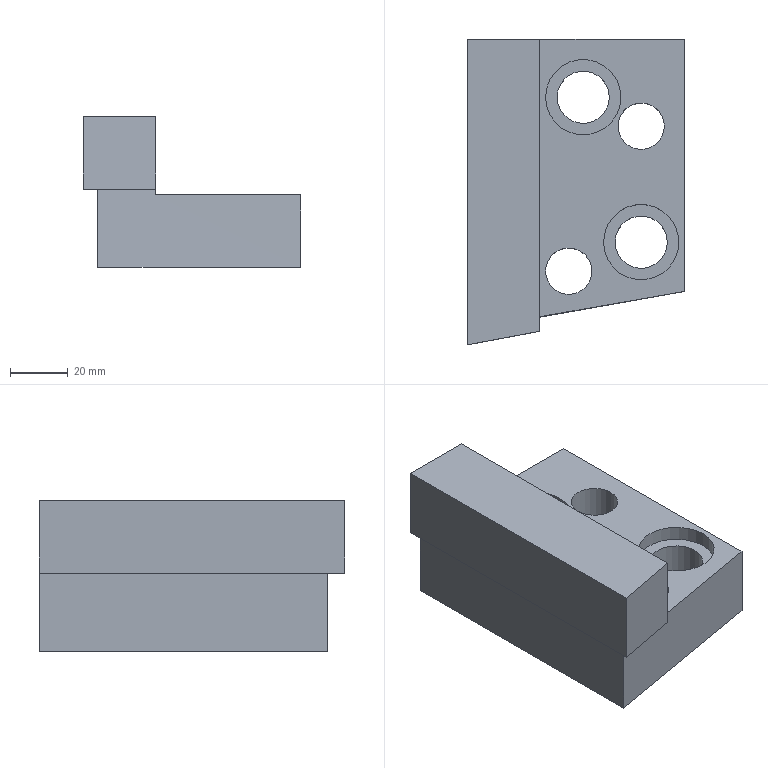Part | NX | features solid 2 | 1 solid | 19 faces | box 75 x 105.467 x 52 mm | volume 205777 mm3 | plane 11 | cylinder 6 | spline 2 | commonest cylinder face diameters 16 x2 18 x2 26 x2
STEP:
#1=CARTESIAN_POINT('',(-221.,545.,-55.));
#2=VERTEX_POINT('',#1);
#3=CARTESIAN_POINT('',(-230.,545.,-55.));
#4=DIRECTION('',(0.,0.,1.));
#5=DIRECTION('',(1.,0.,0.));
#6=AXIS2_PLACEMENT_3D('',#3,#4,#5);
#7=CIRCLE('',#6,9.);
#8=EDGE_CURVE('',#2,#2,#7,.F.);
#9=ORIENTED_EDGE('',*,*,#8,.F.);
#10=EDGE_LOOP('',(#9));
#11=FACE_BOUND('',#10,.T.);
#12=CARTESIAN_POINT('',(-241.,595.,-55.));
#13=VERTEX_POINT('',#12);
#14=CARTESIAN_POINT('',(-250.,595.,-55.));
#15=DIRECTION('',(0.,0.,1.));
#16=DIRECTION('',(1.,0.,0.));
#17=AXIS2_PLACEMENT_3D('',#14,#15,#16);
#18=CIRCLE('',#17,9.);
#19=EDGE_CURVE('',#13,#13,#18,.T.);
#20=ORIENTED_EDGE('',*,*,#19,.T.);
#21=EDGE_LOOP('',(#20));
#22=FACE_BOUND('',#21,.T.);
#23=CARTESIAN_POINT('',(-222.,585.,-55.));
#24=VERTEX_POINT('',#23);
#25=CARTESIAN_POINT('',(-230.,585.,-55.));
#26=DIRECTION('',(0.,0.,1.));
#27=DIRECTION('',(1.,0.,0.));
#28=AXIS2_PLACEMENT_3D('',#25,#26,#27);
#29=CIRCLE('',#28,8.);
#30=EDGE_CURVE('',#24,#24,#29,.T.);
#31=ORIENTED_EDGE('',*,*,#30,.T.);
#32=EDGE_LOOP('',(#31));
#33=FACE_BOUND('',#32,.T.);
#34=CARTESIAN_POINT('',(-215.,528.003,-55.));
#35=VERTEX_POINT('',#34);
#36=CARTESIAN_POINT('',(-215.,615.,-55.));
#37=VERTEX_POINT('',#36);
#38=CARTESIAN_POINT('',(-215.,477.364,-55.));
#39=DIRECTION('',(0.,1.,0.));
#40=VECTOR('',#39,1000.);
#41=LINE('',#38,#40);
#42=EDGE_CURVE('',#35,#37,#41,.T.);
#43=ORIENTED_EDGE('',*,*,#42,.F.);
#44=CARTESIAN_POINT('',(-285.,515.602,-55.));
#45=VERTEX_POINT('',#44);
#46=CARTESIAN_POINT('',(-215.,528.003,-55.));
#47=CARTESIAN_POINT('',(-226.671,525.962,-55.));
#48=CARTESIAN_POINT('',(-250.01,521.86,-55.));
#49=CARTESIAN_POINT('',(-273.364,517.836,-55.));
#50=CARTESIAN_POINT('',(-285.,515.602,-55.));
#51=B_SPLINE_CURVE_WITH_KNOTS('',3,(#46,#47,#48,#49,#50),.UNSPECIFIED.,.F.,.F.,(4,1,4),(0.,0.03555,0.07109),.UNSPECIFIED.);
#52=EDGE_CURVE('',#35,#45,#51,.T.);
#53=ORIENTED_EDGE('',*,*,#52,.T.);
#54=CARTESIAN_POINT('',(-285.,615.,-55.));
#55=VERTEX_POINT('',#54);
#56=CARTESIAN_POINT('',(-285.,474.207,-55.));
#57=DIRECTION('',(0.,1.,0.));
#58=VECTOR('',#57,1000.);
#59=LINE('',#56,#58);
#60=EDGE_CURVE('',#45,#55,#59,.T.);
#61=ORIENTED_EDGE('',*,*,#60,.T.);
#62=CARTESIAN_POINT('',(-277.501,615.,-55.));
#63=DIRECTION('',(-1.,0.,0.));
#64=VECTOR('',#63,1000.);
#65=LINE('',#62,#64);
#66=EDGE_CURVE('',#37,#55,#65,.T.);
#67=ORIENTED_EDGE('',*,*,#66,.F.);
#68=EDGE_LOOP('',(#43,#53,#61,#67));
#69=FACE_BOUND('',#68,.T.);
#70=CARTESIAN_POINT('',(-247.,535.,-55.));
#71=VERTEX_POINT('',#70);
#72=CARTESIAN_POINT('',(-255.,535.,-55.));
#73=DIRECTION('',(0.,0.,1.));
#74=DIRECTION('',(1.,0.,0.));
#75=AXIS2_PLACEMENT_3D('',#72,#73,#74);
#76=CIRCLE('',#75,8.);
#77=EDGE_CURVE('',#71,#71,#76,.F.);
#78=ORIENTED_EDGE('',*,*,#77,.F.);
#79=EDGE_LOOP('',(#78));
#80=FACE_BOUND('',#79,.T.);
#81=CARTESIAN_POINT('',(-277.501,477.364,-55.));
#82=DIRECTION('',(0.,0.,1.));
#83=DIRECTION('',(1.,0.,0.));
#84=AXIS2_PLACEMENT_3D('',#81,#82,#83);
#85=PLANE('',#84);
#86=ADVANCED_FACE('',(#11,#22,#33,#69,#80),#85,.F.);
#87=CARTESIAN_POINT('',(-217.,545.,-30.));
#88=VERTEX_POINT('',#87);
#89=CARTESIAN_POINT('',(-230.,545.,-30.));
#90=DIRECTION('',(0.,0.,1.));
#91=DIRECTION('',(1.,0.,0.));
#92=AXIS2_PLACEMENT_3D('',#89,#90,#91);
#93=CIRCLE('',#92,13.);
#94=EDGE_CURVE('',#88,#88,#93,.F.);
#95=ORIENTED_EDGE('',*,*,#94,.T.);
#96=EDGE_LOOP('',(#95));
#97=FACE_BOUND('',#96,.T.);
#98=CARTESIAN_POINT('',(-215.,528.003,-30.));
#99=VERTEX_POINT('',#98);
#100=CARTESIAN_POINT('',(-265.,519.259,-30.));
#101=VERTEX_POINT('',#100);
#102=CARTESIAN_POINT('',(-215.,528.003,-30.));
#103=CARTESIAN_POINT('',(-231.667,525.088,-30.));
#104=CARTESIAN_POINT('',(-248.333,522.174,-30.));
#105=CARTESIAN_POINT('',(-265.,519.259,-30.));
#106=B_SPLINE_CURVE_WITH_KNOTS('',3,(#102,#103,#104,#105),.UNSPECIFIED.,.F.,.F.,(4,4),(0.,0.05076),.UNSPECIFIED.);
#107=EDGE_CURVE('',#99,#101,#106,.T.);
#108=ORIENTED_EDGE('',*,*,#107,.F.);
#109=CARTESIAN_POINT('',(-215.,615.,-30.));
#110=VERTEX_POINT('',#109);
#111=CARTESIAN_POINT('',(-215.,487.395,-30.));
#112=DIRECTION('',(0.,1.,0.));
#113=VECTOR('',#112,1000.);
#114=LINE('',#111,#113);
#115=EDGE_CURVE('',#99,#110,#114,.T.);
#116=ORIENTED_EDGE('',*,*,#115,.T.);
#117=CARTESIAN_POINT('',(-265.,615.,-30.));
#118=VERTEX_POINT('',#117);
#119=CARTESIAN_POINT('',(-237.5,615.,-30.));
#120=DIRECTION('',(-1.,0.,0.));
#121=VECTOR('',#120,1000.);
#122=LINE('',#119,#121);
#123=EDGE_CURVE('',#110,#118,#122,.T.);
#124=ORIENTED_EDGE('',*,*,#123,.T.);
#125=CARTESIAN_POINT('',(-265.,487.395,-30.));
#126=DIRECTION('',(0.,1.,0.));
#127=VECTOR('',#126,1000.);
#128=LINE('',#125,#127);
#129=EDGE_CURVE('',#101,#118,#128,.T.);
#130=ORIENTED_EDGE('',*,*,#129,.F.);
#131=EDGE_LOOP('',(#108,#116,#124,#130));
#132=FACE_BOUND('',#131,.T.);
#133=CARTESIAN_POINT('',(-222.,585.,-30.));
#134=VERTEX_POINT('',#133);
#135=CARTESIAN_POINT('',(-230.,585.,-30.));
#136=DIRECTION('',(0.,0.,1.));
#137=DIRECTION('',(1.,0.,0.));
#138=AXIS2_PLACEMENT_3D('',#135,#136,#137);
#139=CIRCLE('',#138,8.);
#140=EDGE_CURVE('',#134,#134,#139,.T.);
#141=ORIENTED_EDGE('',*,*,#140,.F.);
#142=EDGE_LOOP('',(#141));
#143=FACE_BOUND('',#142,.T.);
#144=CARTESIAN_POINT('',(-237.,595.,-30.));
#145=VERTEX_POINT('',#144);
#146=CARTESIAN_POINT('',(-250.,595.,-30.));
#147=DIRECTION('',(0.,0.,1.));
#148=DIRECTION('',(1.,0.,0.));
#149=AXIS2_PLACEMENT_3D('',#146,#147,#148);
#150=CIRCLE('',#149,13.);
#151=EDGE_CURVE('',#145,#145,#150,.T.);
#152=ORIENTED_EDGE('',*,*,#151,.F.);
#153=EDGE_LOOP('',(#152));
#154=FACE_BOUND('',#153,.T.);
#155=CARTESIAN_POINT('',(-247.,535.,-30.));
#156=VERTEX_POINT('',#155);
#157=CARTESIAN_POINT('',(-255.,535.,-30.));
#158=DIRECTION('',(0.,0.,1.));
#159=DIRECTION('',(1.,0.,0.));
#160=AXIS2_PLACEMENT_3D('',#157,#158,#159);
#161=CIRCLE('',#160,8.);
#162=EDGE_CURVE('',#156,#156,#161,.F.);
#163=ORIENTED_EDGE('',*,*,#162,.T.);
#164=EDGE_LOOP('',(#163));
#165=FACE_BOUND('',#164,.T.);
#166=CARTESIAN_POINT('',(-237.5,487.395,-30.));
#167=DIRECTION('',(0.,0.,1.));
#168=DIRECTION('',(1.,0.,0.));
#169=AXIS2_PLACEMENT_3D('',#166,#167,#168);
#170=PLANE('',#169);
#171=ADVANCED_FACE('',(#97,#132,#143,#154,#165),#170,.T.);
#172=CARTESIAN_POINT('',(-217.,545.,-35.));
#173=VERTEX_POINT('',#172);
#174=CARTESIAN_POINT('',(-230.,545.,-35.));
#175=DIRECTION('',(0.,0.,1.));
#176=DIRECTION('',(1.,0.,0.));
#177=AXIS2_PLACEMENT_3D('',#174,#175,#176);
#178=CIRCLE('',#177,13.);
#179=EDGE_CURVE('',#173,#173,#178,.T.);
#180=ORIENTED_EDGE('',*,*,#179,.T.);
#181=EDGE_LOOP('',(#180));
#182=FACE_BOUND('',#181,.T.);
#183=CARTESIAN_POINT('',(-221.,545.,-35.));
#184=VERTEX_POINT('',#183);
#185=CARTESIAN_POINT('',(-230.,545.,-35.));
#186=DIRECTION('',(0.,0.,1.));
#187=DIRECTION('',(1.,0.,0.));
#188=AXIS2_PLACEMENT_3D('',#185,#186,#187);
#189=CIRCLE('',#188,9.);
#190=EDGE_CURVE('',#184,#184,#189,.F.);
#191=ORIENTED_EDGE('',*,*,#190,.T.);
#192=EDGE_LOOP('',(#191));
#193=FACE_BOUND('',#192,.T.);
#194=CARTESIAN_POINT('',(-230.,545.,-35.));
#195=DIRECTION('',(0.,0.,1.));
#196=DIRECTION('',(1.,0.,0.));
#197=AXIS2_PLACEMENT_3D('',#194,#195,#196);
#198=PLANE('',#197);
#199=ADVANCED_FACE('',(#182,#193),#198,.T.);
#200=CARTESIAN_POINT('',(-290.,509.533,-3.));
#201=VERTEX_POINT('',#200);
#202=CARTESIAN_POINT('',(-290.,509.533,-28.));
#203=VERTEX_POINT('',#202);
#204=CARTESIAN_POINT('',(-290.,509.533,100.));
#205=DIRECTION('',(0.,0.,-1.));
#206=VECTOR('',#205,1000.);
#207=LINE('',#204,#206);
#208=EDGE_CURVE('',#201,#203,#207,.T.);
#209=ORIENTED_EDGE('',*,*,#208,.F.);
#210=CARTESIAN_POINT('',(-290.,615.,-3.));
#211=VERTEX_POINT('',#210);
#212=CARTESIAN_POINT('',(-290.,474.207,-3.));
#213=DIRECTION('',(0.,1.,0.));
#214=VECTOR('',#213,1000.);
#215=LINE('',#212,#214);
#216=EDGE_CURVE('',#201,#211,#215,.T.);
#217=ORIENTED_EDGE('',*,*,#216,.T.);
#218=CARTESIAN_POINT('',(-290.,615.,-28.));
#219=VERTEX_POINT('',#218);
#220=CARTESIAN_POINT('',(-290.,615.,-53.));
#221=DIRECTION('',(0.,0.,1.));
#222=VECTOR('',#221,1000.);
#223=LINE('',#220,#222);
#224=EDGE_CURVE('',#219,#211,#223,.T.);
#225=ORIENTED_EDGE('',*,*,#224,.F.);
#226=CARTESIAN_POINT('',(-290.,474.207,-28.));
#227=DIRECTION('',(0.,-1.,0.));
#228=VECTOR('',#227,1000.);
#229=LINE('',#226,#228);
#230=EDGE_CURVE('',#203,#219,#229,.F.);
#231=ORIENTED_EDGE('',*,*,#230,.F.);
#232=EDGE_LOOP('',(#209,#217,#225,#231));
#233=FACE_BOUND('',#232,.T.);
#234=CARTESIAN_POINT('',(-290.,474.207,-53.));
#235=DIRECTION('',(1.,0.,0.));
#236=DIRECTION('',(0.,0.,-1.));
#237=AXIS2_PLACEMENT_3D('',#234,#235,#236);
#238=PLANE('',#237);
#239=ADVANCED_FACE('',(#233),#238,.F.);
#240=CARTESIAN_POINT('',(-265.,519.259,-28.));
#241=VERTEX_POINT('',#240);
#242=CARTESIAN_POINT('',(-265.,514.183,-28.));
#243=VERTEX_POINT('',#242);
#244=CARTESIAN_POINT('',(-265.,480.509,-28.));
#245=DIRECTION('',(0.,-1.,0.));
#246=VECTOR('',#245,1000.);
#247=LINE('',#244,#246);
#248=EDGE_CURVE('',#241,#243,#247,.T.);
#249=ORIENTED_EDGE('',*,*,#248,.F.);
#250=CARTESIAN_POINT('',(-265.,519.259,-78.));
#251=DIRECTION('',(0.,0.,-1.));
#252=VECTOR('',#251,1000.);
#253=LINE('',#250,#252);
#254=EDGE_CURVE('',#101,#241,#253,.F.);
#255=ORIENTED_EDGE('',*,*,#254,.F.);
#256=ORIENTED_EDGE('',*,*,#129,.T.);
#257=CARTESIAN_POINT('',(-265.,615.,-3.));
#258=VERTEX_POINT('',#257);
#259=CARTESIAN_POINT('',(-265.,615.,-53.));
#260=DIRECTION('',(0.,0.,1.));
#261=VECTOR('',#260,1000.);
#262=LINE('',#259,#261);
#263=EDGE_CURVE('',#118,#258,#262,.T.);
#264=ORIENTED_EDGE('',*,*,#263,.T.);
#265=CARTESIAN_POINT('',(-265.,514.183,-3.));
#266=VERTEX_POINT('',#265);
#267=CARTESIAN_POINT('',(-265.,480.509,-3.));
#268=DIRECTION('',(0.,1.,0.));
#269=VECTOR('',#268,1000.);
#270=LINE('',#267,#269);
#271=EDGE_CURVE('',#266,#258,#270,.T.);
#272=ORIENTED_EDGE('',*,*,#271,.F.);
#273=CARTESIAN_POINT('',(-265.,514.183,100.));
#274=DIRECTION('',(0.,0.,-1.));
#275=VECTOR('',#274,1000.);
#276=LINE('',#273,#275);
#277=EDGE_CURVE('',#266,#243,#276,.T.);
#278=ORIENTED_EDGE('',*,*,#277,.T.);
#279=EDGE_LOOP('',(#249,#255,#256,#264,#272,#278));
#280=FACE_BOUND('',#279,.T.);
#281=CARTESIAN_POINT('',(-265.,480.509,-53.));
#282=DIRECTION('',(1.,0.,0.));
#283=DIRECTION('',(0.,0.,-1.));
#284=AXIS2_PLACEMENT_3D('',#281,#282,#283);
#285=PLANE('',#284);
#286=ADVANCED_FACE('',(#280),#285,.T.);
#287=ORIENTED_EDGE('',*,*,#216,.F.);
#288=CARTESIAN_POINT('',(314.417,604.257,-3.));
#289=CARTESIAN_POINT('',(313.456,603.513,-3.));
#290=CARTESIAN_POINT('',(311.997,602.42,-3.));
#291=CARTESIAN_POINT('',(310.125,600.866,-3.));
#292=CARTESIAN_POINT('',(308.006,599.638,-3.));
#293=CARTESIAN_POINT('',(304.985,599.087,-3.));
#294=CARTESIAN_POINT('',(297.755,598.23,-3.));
#295=CARTESIAN_POINT('',(282.167,595.571,-3.));
#296=CARTESIAN_POINT('',(258.333,590.865,-3.));
#297=CARTESIAN_POINT('',(229.601,585.825,-3.));
#298=CARTESIAN_POINT('',(200.669,582.121,-3.));
#299=CARTESIAN_POINT('',(171.683,578.904,-3.));
#300=CARTESIAN_POINT('',(142.767,575.084,-3.));
#301=CARTESIAN_POINT('',(113.981,570.414,-3.));
#302=CARTESIAN_POINT('',(85.244,565.431,-3.));
#303=CARTESIAN_POINT('',(56.452,560.795,-3.));
#304=CARTESIAN_POINT('',(27.599,556.541,-3.));
#305=CARTESIAN_POINT('',(-1.295,552.585,-3.));
#306=CARTESIAN_POINT('',(-39.83,547.381,-3.));
#307=CARTESIAN_POINT('',(-87.902,540.194,-3.));
#308=CARTESIAN_POINT('',(-145.572,531.452,-3.));
#309=CARTESIAN_POINT('',(-203.407,523.885,-3.));
#310=CARTESIAN_POINT('',(-261.096,515.298,-3.));
#311=CARTESIAN_POINT('',(-318.405,504.143,-3.));
#312=CARTESIAN_POINT('',(-374.806,489.184,-3.));
#313=CARTESIAN_POINT('',(-420.452,472.38,-3.));
#314=CARTESIAN_POINT('',(-456.779,458.517,-3.));
#315=CARTESIAN_POINT('',(-484.05,448.183,-3.));
#316=CARTESIAN_POINT('',(-511.125,437.331,-3.));
#317=CARTESIAN_POINT('',(-546.415,420.942,-3.));
#318=CARTESIAN_POINT('',(-571.409,405.8,-3.));
#319=CARTESIAN_POINT('',(-587.555,394.969,-3.));
#320=B_SPLINE_CURVE_WITH_KNOTS('',3,(#288,#289,#290,#291,#292,#293,#294,#295,#296,#297,#298,#299,#300,#301,#302,#303,#304,#305,#306,#307,#308,#309,#310,#311,#312,#313,#314,#315,#316,#317,#318,#319),.UNSPECIFIED.,.F.,.F.,(4,1,1,1,1,1,1,1,1,1,1,1,1,1,1,1,1,1,1,1,1,1,1,1,1,1,1,1,1,4),(0.,0.002796,0.004195,0.005593,0.008389,0.01119,0.02237,0.04474,0.06711,0.08948,0.1119,0.1342,0.1566,0.179,0.2013,0.2237,0.2461,0.2684,0.3132,0.3579,0.4027,0.4474,0.4922,0.5369,0.5816,0.604,0.6264,0.6488,0.6711,0.7159),.UNSPECIFIED.);
#321=EDGE_CURVE('',#201,#266,#320,.F.);
#322=ORIENTED_EDGE('',*,*,#321,.T.);
#323=ORIENTED_EDGE('',*,*,#271,.T.);
#324=CARTESIAN_POINT('',(-277.501,615.,-3.));
#325=DIRECTION('',(-1.,0.,0.));
#326=VECTOR('',#325,1000.);
#327=LINE('',#324,#326);
#328=EDGE_CURVE('',#258,#211,#327,.T.);
#329=ORIENTED_EDGE('',*,*,#328,.T.);
#330=EDGE_LOOP('',(#287,#322,#323,#329));
#331=FACE_BOUND('',#330,.T.);
#332=CARTESIAN_POINT('',(-277.501,477.364,-3.));
#333=DIRECTION('',(0.,0.,1.));
#334=DIRECTION('',(1.,0.,0.));
#335=AXIS2_PLACEMENT_3D('',#332,#333,#334);
#336=PLANE('',#335);
#337=ADVANCED_FACE('',(#331),#336,.T.);
#338=CARTESIAN_POINT('',(-285.,515.602,-28.));
#339=VERTEX_POINT('',#338);
#340=CARTESIAN_POINT('',(-285.,515.602,-78.));
#341=DIRECTION('',(0.,0.,-1.));
#342=VECTOR('',#341,1000.);
#343=LINE('',#340,#342);
#344=EDGE_CURVE('',#339,#45,#343,.T.);
#345=ORIENTED_EDGE('',*,*,#344,.F.);
#346=CARTESIAN_POINT('',(-285.,615.,-28.));
#347=VERTEX_POINT('',#346);
#348=CARTESIAN_POINT('',(-285.,474.207,-28.));
#349=DIRECTION('',(0.,1.,0.));
#350=VECTOR('',#349,1000.);
#351=LINE('',#348,#350);
#352=EDGE_CURVE('',#339,#347,#351,.T.);
#353=ORIENTED_EDGE('',*,*,#352,.T.);
#354=CARTESIAN_POINT('',(-285.,615.,-53.));
#355=DIRECTION('',(0.,0.,1.));
#356=VECTOR('',#355,1000.);
#357=LINE('',#354,#356);
#358=EDGE_CURVE('',#55,#347,#357,.T.);
#359=ORIENTED_EDGE('',*,*,#358,.F.);
#360=ORIENTED_EDGE('',*,*,#60,.F.);
#361=EDGE_LOOP('',(#345,#353,#359,#360));
#362=FACE_BOUND('',#361,.T.);
#363=CARTESIAN_POINT('',(-285.,474.207,-28.));
#364=DIRECTION('',(-1.,0.,0.));
#365=DIRECTION('',(0.,0.,1.));
#366=AXIS2_PLACEMENT_3D('',#363,#364,#365);
#367=PLANE('',#366);
#368=ADVANCED_FACE('',(#362),#367,.T.);
#369=CARTESIAN_POINT('',(-215.,528.003,-78.));
#370=DIRECTION('',(0.,0.,-1.));
#371=VECTOR('',#370,1000.);
#372=LINE('',#369,#371);
#373=EDGE_CURVE('',#35,#99,#372,.F.);
#374=ORIENTED_EDGE('',*,*,#373,.F.);
#375=ORIENTED_EDGE('',*,*,#42,.T.);
#376=CARTESIAN_POINT('',(-215.,615.,-53.));
#377=DIRECTION('',(0.,0.,1.));
#378=VECTOR('',#377,1000.);
#379=LINE('',#376,#378);
#380=EDGE_CURVE('',#37,#110,#379,.T.);
#381=ORIENTED_EDGE('',*,*,#380,.T.);
#382=ORIENTED_EDGE('',*,*,#115,.F.);
#383=EDGE_LOOP('',(#374,#375,#381,#382));
#384=FACE_BOUND('',#383,.T.);
#385=CARTESIAN_POINT('',(-215.,494.281,-53.));
#386=DIRECTION('',(1.,0.,0.));
#387=DIRECTION('',(0.,0.,-1.));
#388=AXIS2_PLACEMENT_3D('',#385,#386,#387);
#389=PLANE('',#388);
#390=ADVANCED_FACE('',(#384),#389,.T.);
#391=ORIENTED_EDGE('',*,*,#19,.F.);
#392=EDGE_LOOP('',(#391));
#393=FACE_BOUND('',#392,.T.);
#394=CARTESIAN_POINT('',(-241.,595.,-35.));
#395=VERTEX_POINT('',#394);
#396=CARTESIAN_POINT('',(-250.,595.,-35.));
#397=DIRECTION('',(0.,0.,1.));
#398=DIRECTION('',(1.,0.,0.));
#399=AXIS2_PLACEMENT_3D('',#396,#397,#398);
#400=CIRCLE('',#399,9.);
#401=EDGE_CURVE('',#395,#395,#400,.F.);
#402=ORIENTED_EDGE('',*,*,#401,.F.);
#403=EDGE_LOOP('',(#402));
#404=FACE_BOUND('',#403,.T.);
#405=CARTESIAN_POINT('',(-250.,595.,-60.));
#406=DIRECTION('',(0.,0.,1.));
#407=DIRECTION('',(1.,0.,0.));
#408=AXIS2_PLACEMENT_3D('',#405,#406,#407);
#409=CYLINDRICAL_SURFACE('',#408,9.);
#410=ADVANCED_FACE('',(#393,#404),#409,.F.);
#411=CARTESIAN_POINT('',(-290.,615.,-28.));
#412=DIRECTION('',(-1.,0.,0.));
#413=VECTOR('',#412,1000.);
#414=LINE('',#411,#413);
#415=EDGE_CURVE('',#219,#347,#414,.F.);
#416=ORIENTED_EDGE('',*,*,#415,.F.);
#417=ORIENTED_EDGE('',*,*,#224,.T.);
#418=ORIENTED_EDGE('',*,*,#328,.F.);
#419=ORIENTED_EDGE('',*,*,#263,.F.);
#420=ORIENTED_EDGE('',*,*,#123,.F.);
#421=ORIENTED_EDGE('',*,*,#380,.F.);
#422=ORIENTED_EDGE('',*,*,#66,.T.);
#423=ORIENTED_EDGE('',*,*,#358,.T.);
#424=EDGE_LOOP('',(#416,#417,#418,#419,#420,#421,#422,#423));
#425=FACE_BOUND('',#424,.T.);
#426=CARTESIAN_POINT('',(-265.,615.,-53.));
#427=DIRECTION('',(0.,1.,0.));
#428=DIRECTION('',(0.,0.,1.));
#429=AXIS2_PLACEMENT_3D('',#426,#427,#428);
#430=PLANE('',#429);
#431=ADVANCED_FACE('',(#425),#430,.T.);
#432=ORIENTED_EDGE('',*,*,#352,.F.);
#433=CARTESIAN_POINT('',(-285.,515.602,-28.));
#434=CARTESIAN_POINT('',(-278.341,516.88,-28.));
#435=CARTESIAN_POINT('',(-271.648,518.096,-28.));
#436=CARTESIAN_POINT('',(-265.,519.259,-28.));
#437=B_SPLINE_CURVE_WITH_KNOTS('',3,(#433,#434,#435,#436),.UNSPECIFIED.,.F.,.F.,(4,4),(0.2381,1.034),.UNSPECIFIED.);
#438=EDGE_CURVE('',#339,#241,#437,.T.);
#439=ORIENTED_EDGE('',*,*,#438,.T.);
#440=ORIENTED_EDGE('',*,*,#248,.T.);
#441=CARTESIAN_POINT('',(314.417,604.257,-28.));
#442=CARTESIAN_POINT('',(313.456,603.513,-28.));
#443=CARTESIAN_POINT('',(311.997,602.42,-28.));
#444=CARTESIAN_POINT('',(310.125,600.866,-28.));
#445=CARTESIAN_POINT('',(308.006,599.638,-28.));
#446=CARTESIAN_POINT('',(304.985,599.087,-28.));
#447=CARTESIAN_POINT('',(297.755,598.23,-28.));
#448=CARTESIAN_POINT('',(282.167,595.571,-28.));
#449=CARTESIAN_POINT('',(258.333,590.865,-28.));
#450=CARTESIAN_POINT('',(229.601,585.825,-28.));
#451=CARTESIAN_POINT('',(200.669,582.121,-28.));
#452=CARTESIAN_POINT('',(171.683,578.904,-28.));
#453=CARTESIAN_POINT('',(142.767,575.084,-28.));
#454=CARTESIAN_POINT('',(113.981,570.414,-28.));
#455=CARTESIAN_POINT('',(85.244,565.431,-28.));
#456=CARTESIAN_POINT('',(56.452,560.795,-28.));
#457=CARTESIAN_POINT('',(27.599,556.541,-28.));
#458=CARTESIAN_POINT('',(-1.295,552.585,-28.));
#459=CARTESIAN_POINT('',(-39.83,547.381,-28.));
#460=CARTESIAN_POINT('',(-87.902,540.194,-28.));
#461=CARTESIAN_POINT('',(-145.572,531.452,-28.));
#462=CARTESIAN_POINT('',(-203.407,523.885,-28.));
#463=CARTESIAN_POINT('',(-261.096,515.298,-28.));
#464=CARTESIAN_POINT('',(-318.405,504.143,-28.));
#465=CARTESIAN_POINT('',(-374.806,489.184,-28.));
#466=CARTESIAN_POINT('',(-420.452,472.38,-28.));
#467=CARTESIAN_POINT('',(-456.779,458.517,-28.));
#468=CARTESIAN_POINT('',(-484.05,448.183,-28.));
#469=CARTESIAN_POINT('',(-511.125,437.331,-28.));
#470=CARTESIAN_POINT('',(-546.415,420.942,-28.));
#471=CARTESIAN_POINT('',(-571.409,405.8,-28.));
#472=CARTESIAN_POINT('',(-587.555,394.969,-28.));
#473=B_SPLINE_CURVE_WITH_KNOTS('',3,(#441,#442,#443,#444,#445,#446,#447,#448,#449,#450,#451,#452,#453,#454,#455,#456,#457,#458,#459,#460,#461,#462,#463,#464,#465,#466,#467,#468,#469,#470,#471,#472),.UNSPECIFIED.,.F.,.F.,(4,1,1,1,1,1,1,1,1,1,1,1,1,1,1,1,1,1,1,1,1,1,1,1,1,1,1,1,1,4),(0.,0.002796,0.004195,0.005593,0.008389,0.01119,0.02237,0.04474,0.06711,0.08948,0.1119,0.1342,0.1566,0.179,0.2013,0.2237,0.2461,0.2684,0.3132,0.3579,0.4027,0.4474,0.4922,0.5369,0.5816,0.604,0.6264,0.6488,0.6711,0.7159),.UNSPECIFIED.);
#474=EDGE_CURVE('',#203,#243,#473,.F.);
#475=ORIENTED_EDGE('',*,*,#474,.F.);
#476=ORIENTED_EDGE('',*,*,#230,.T.);
#477=ORIENTED_EDGE('',*,*,#415,.T.);
#478=EDGE_LOOP('',(#432,#439,#440,#475,#476,#477));
#479=FACE_BOUND('',#478,.T.);
#480=CARTESIAN_POINT('',(-290.,474.207,-28.));
#481=DIRECTION('',(0.,0.,1.));
#482=DIRECTION('',(1.,0.,0.));
#483=AXIS2_PLACEMENT_3D('',#480,#481,#482);
#484=PLANE('',#483);
#485=ADVANCED_FACE('',(#479),#484,.F.);
#486=ORIENTED_EDGE('',*,*,#140,.T.);
#487=EDGE_LOOP('',(#486));
#488=FACE_BOUND('',#487,.T.);
#489=ORIENTED_EDGE('',*,*,#30,.F.);
#490=EDGE_LOOP('',(#489));
#491=FACE_BOUND('',#490,.T.);
#492=CARTESIAN_POINT('',(-230.,585.,-60.));
#493=DIRECTION('',(0.,0.,1.));
#494=DIRECTION('',(1.,0.,0.));
#495=AXIS2_PLACEMENT_3D('',#492,#493,#494);
#496=CYLINDRICAL_SURFACE('',#495,8.);
#497=ADVANCED_FACE('',(#488,#491),#496,.F.);
#498=CARTESIAN_POINT('',(-237.,595.,-35.));
#499=VERTEX_POINT('',#498);
#500=CARTESIAN_POINT('',(-250.,595.,-35.));
#501=DIRECTION('',(0.,0.,1.));
#502=DIRECTION('',(1.,0.,0.));
#503=AXIS2_PLACEMENT_3D('',#500,#501,#502);
#504=CIRCLE('',#503,13.);
#505=EDGE_CURVE('',#499,#499,#504,.T.);
#506=ORIENTED_EDGE('',*,*,#505,.T.);
#507=EDGE_LOOP('',(#506));
#508=FACE_BOUND('',#507,.T.);
#509=ORIENTED_EDGE('',*,*,#401,.T.);
#510=EDGE_LOOP('',(#509));
#511=FACE_BOUND('',#510,.T.);
#512=CARTESIAN_POINT('',(-250.,595.,-35.));
#513=DIRECTION('',(0.,0.,1.));
#514=DIRECTION('',(1.,0.,0.));
#515=AXIS2_PLACEMENT_3D('',#512,#513,#514);
#516=PLANE('',#515);
#517=ADVANCED_FACE('',(#508,#511),#516,.T.);
#518=ORIENTED_EDGE('',*,*,#505,.F.);
#519=EDGE_LOOP('',(#518));
#520=FACE_BOUND('',#519,.T.);
#521=ORIENTED_EDGE('',*,*,#151,.T.);
#522=EDGE_LOOP('',(#521));
#523=FACE_BOUND('',#522,.T.);
#524=CARTESIAN_POINT('',(-250.,595.,-35.));
#525=DIRECTION('',(0.,0.,1.));
#526=DIRECTION('',(1.,0.,0.));
#527=AXIS2_PLACEMENT_3D('',#524,#525,#526);
#528=CYLINDRICAL_SURFACE('',#527,13.);
#529=ADVANCED_FACE('',(#520,#523),#528,.F.);
#530=ORIENTED_EDGE('',*,*,#474,.T.);
#531=ORIENTED_EDGE('',*,*,#277,.F.);
#532=ORIENTED_EDGE('',*,*,#321,.F.);
#533=ORIENTED_EDGE('',*,*,#208,.T.);
#534=EDGE_LOOP('',(#530,#531,#532,#533));
#535=FACE_BOUND('',#534,.T.);
#536=CARTESIAN_POINT('',(-265.,514.183,-3.));
#537=CARTESIAN_POINT('',(-265.,514.183,-28.));
#538=CARTESIAN_POINT('',(-273.349,512.723,-3.));
#539=CARTESIAN_POINT('',(-273.349,512.723,-28.));
#540=CARTESIAN_POINT('',(-281.685,511.178,-3.));
#541=CARTESIAN_POINT('',(-281.685,511.178,-28.));
#542=CARTESIAN_POINT('',(-290.,509.533,-3.));
#543=CARTESIAN_POINT('',(-290.,509.533,-28.));
#544=B_SPLINE_SURFACE_WITH_KNOTS('',3,1,((#536,#537),(#538,#539),(#540,#541),(#542,#543)),.SURF_OF_LINEAR_EXTRUSION.,.F.,.F.,.F.,(4,4),(2,2),(0.4505,0.47),(0.,1.),.PIECEWISE_BEZIER_KNOTS.);
#545=ADVANCED_FACE('',(#535),#544,.T.);
#546=ORIENTED_EDGE('',*,*,#344,.T.);
#547=ORIENTED_EDGE('',*,*,#52,.F.);
#548=ORIENTED_EDGE('',*,*,#373,.T.);
#549=ORIENTED_EDGE('',*,*,#107,.T.);
#550=ORIENTED_EDGE('',*,*,#254,.T.);
#551=ORIENTED_EDGE('',*,*,#438,.F.);
#552=EDGE_LOOP('',(#546,#547,#548,#549,#550,#551));
#553=FACE_BOUND('',#552,.T.);
#554=CARTESIAN_POINT('',(-285.,515.602,-28.));
#555=CARTESIAN_POINT('',(-285.,515.602,-55.));
#556=CARTESIAN_POINT('',(-273.323,517.843,-28.));
#557=CARTESIAN_POINT('',(-273.323,517.843,-55.));
#558=CARTESIAN_POINT('',(-249.955,521.87,-28.));
#559=CARTESIAN_POINT('',(-249.955,521.87,-55.));
#560=CARTESIAN_POINT('',(-226.657,525.964,-28.));
#561=CARTESIAN_POINT('',(-226.657,525.964,-55.));
#562=CARTESIAN_POINT('',(-215.,528.003,-28.));
#563=CARTESIAN_POINT('',(-215.,528.003,-55.));
#564=B_SPLINE_SURFACE_WITH_KNOTS('',3,1,((#554,#555),(#556,#557),(#558,#559),(#560,#561),(#562,#563)),.SURF_OF_LINEAR_EXTRUSION.,.F.,.F.,.F.,(4,1,4),(2,2),(0.2381,1.634,3.031),(0.,1.),.UNSPECIFIED.);
#565=ADVANCED_FACE('',(#553),#564,.F.);
#566=ORIENTED_EDGE('',*,*,#94,.F.);
#567=EDGE_LOOP('',(#566));
#568=FACE_BOUND('',#567,.T.);
#569=ORIENTED_EDGE('',*,*,#179,.F.);
#570=EDGE_LOOP('',(#569));
#571=FACE_BOUND('',#570,.T.);
#572=CARTESIAN_POINT('',(-230.,545.,165.));
#573=DIRECTION('',(0.,0.,-1.));
#574=DIRECTION('',(-1.,0.,0.));
#575=AXIS2_PLACEMENT_3D('',#572,#573,#574);
#576=CYLINDRICAL_SURFACE('',#575,13.);
#577=ADVANCED_FACE('',(#568,#571),#576,.F.);
#578=ORIENTED_EDGE('',*,*,#190,.F.);
#579=EDGE_LOOP('',(#578));
#580=FACE_BOUND('',#579,.T.);
#581=ORIENTED_EDGE('',*,*,#8,.T.);
#582=EDGE_LOOP('',(#581));
#583=FACE_BOUND('',#582,.T.);
#584=CARTESIAN_POINT('',(-230.,545.,-135.));
#585=DIRECTION('',(0.,0.,1.));
#586=DIRECTION('',(1.,0.,0.));
#587=AXIS2_PLACEMENT_3D('',#584,#585,#586);
#588=CYLINDRICAL_SURFACE('',#587,9.);
#589=ADVANCED_FACE('',(#580,#583),#588,.F.);
#590=ORIENTED_EDGE('',*,*,#162,.F.);
#591=EDGE_LOOP('',(#590));
#592=FACE_BOUND('',#591,.T.);
#593=ORIENTED_EDGE('',*,*,#77,.T.);
#594=EDGE_LOOP('',(#593));
#595=FACE_BOUND('',#594,.T.);
#596=CARTESIAN_POINT('',(-255.,535.,170.));
#597=DIRECTION('',(0.,0.,-1.));
#598=DIRECTION('',(-1.,0.,0.));
#599=AXIS2_PLACEMENT_3D('',#596,#597,#598);
#600=CYLINDRICAL_SURFACE('',#599,8.);
#601=ADVANCED_FACE('',(#592,#595),#600,.F.);
#602=CLOSED_SHELL('',(#86,#171,#199,#239,#286,#337,#368,#390,#410,#431,#485,#497,#517,#529,#545,#565,#577,#589,#601));
#603=MANIFOLD_SOLID_BREP('',#602);
#604=(LENGTH_UNIT()NAMED_UNIT(*)SI_UNIT(.MILLI.,.METRE.));
#605=UNCERTAINTY_MEASURE_WITH_UNIT(LENGTH_MEASURE(0.0508),#604,'','');
#606=(NAMED_UNIT(*)PLANE_ANGLE_UNIT()SI_UNIT($,.RADIAN.));
#607=(NAMED_UNIT(*)SI_UNIT($,.STERADIAN.)SOLID_ANGLE_UNIT());
#608=(GEOMETRIC_REPRESENTATION_CONTEXT(3)GLOBAL_UNCERTAINTY_ASSIGNED_CONTEXT((#605))GLOBAL_UNIT_ASSIGNED_CONTEXT((#604,#606,#607))REPRESENTATION_CONTEXT('',''));
#609=ADVANCED_BREP_SHAPE_REPRESENTATION('',(#603),#608);